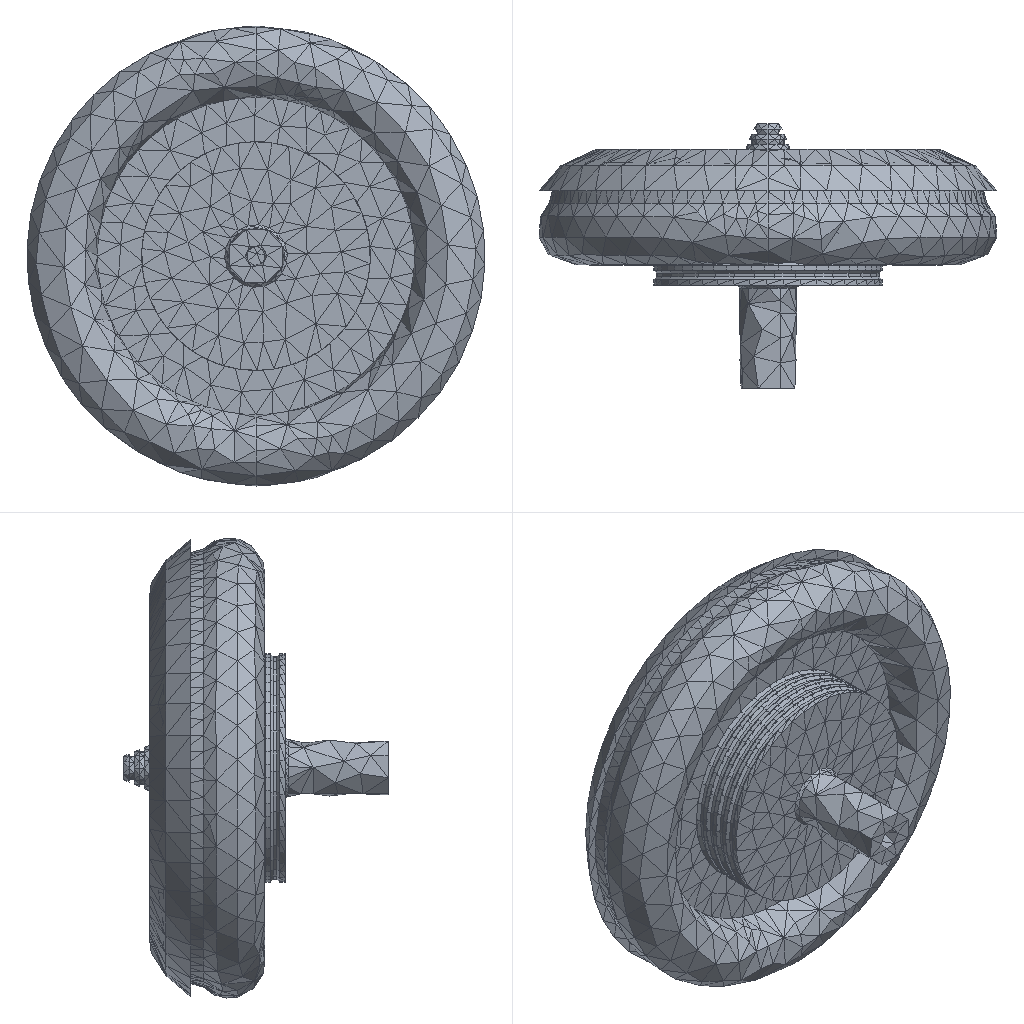Simulation study | ansys workbench
Set-up summary:
category,name,step,type,value,unit,region
solver,ansys_workbench
units,mm-N-s-tonne (MPa),,stated,"/units,MPA"
analysis,LS1,,modal,method=lanb; n_modes=16
load_step,LS1,LS1,modal
mesh,nodes,,,33011
mesh,elements,,,20069
element_type,SOLID187,,,10384
element_type,TARGE170,,,3950
element_type,CONTA174,,,3950
element_type,SOLID186,,,1785
material,Structural Steel,,E,200000,tonne s^-2 mm^-1
material,Structural Steel,,nu,0.3
material,Structural Steel,,density,7.85e-09,tonne mm^-3
material,Structural Steel,,conductivity,60.5,tonne mm s^-3 C^-1
material,Structural Steel,,specific_heat,4.34e+08,mm^2 s^-2 C^-1
material,Structural Steel,,cte,1.2e-05,C^-1
material,Structural Steel,,permeability,10000
material,Structural Steel,,resistivity,0.00017,ohm mm
bc,Fixed Supports,model,fixed,[dofs=ALL],,_FIXEDSU
contact,Contact Region,,bonded (always),element=CONTA174
contact,Contact Region 2,,bonded (always),element=CONTA174
contact,Contact Region 3,,bonded (always),element=CONTA174
contact,Contact Region 4,,bonded (always),element=CONTA174
contact,Contact Region 5,,bonded (always),element=CONTA174
contact,Contact Region 6,,bonded (always),element=CONTA174
contact,Contact Region 7,,bonded (always),element=CONTA174
contact,Contact Region 8,,bonded (always),element=CONTA174
contact,Contact Region 9,,bonded (always),element=CONTA174
contact,Contact Region 10,,bonded (always),element=CONTA174
contact,Contact Region 11,,bonded (always),element=CONTA174
contact,Contact Region 12,,bonded (always),element=CONTA174
contact,Contact Region 13,,bonded (always),element=CONTA174
contact,Contact Region 14,,bonded (always),element=CONTA174
contact,Contact Region 15,,bonded (always),element=CONTA174
contact,Contact Region 16,,bonded (always),element=CONTA174
contact,Contact Region 17,,bonded (always),element=CONTA174
contact,Contact Region 18,,bonded (always),element=CONTA174
contact,Contact Region 19,,bonded (always),element=CONTA174
named_set,_FIXEDSU,,node,71
Ansys APDL input file, long lists of numbers shortened:
/batch
/config,noeldb,1     ! force off writing results to database
*get,_wallstrt,active,,time,wall
! ANSYS input file written by Workbench version 2022 R1
! File used for geometry attach:
/title,wbnew--__ (B5)
! ****** Begin Custom Load Command Snippet ******
/COM, ACT Extensions:
/COM,     LSDYNA, 2021.1
/COM,
! ****** End   Custom Load Command Snippet ******
*DIM,_wb_ProjectScratch_dir,string,248
_wb_ProjectScratch_dir(1) = ''
*DIM,_wb_SolverFiles_dir,string,248
_wb_SolverFiles_dir(1) = ''
*DIM,_wb_userfiles_dir,string,248
_wb_userfiles_dir(1) = ''
/com,--- Data in consistent NMM units. See Solving Units in the help system for more information.
/units,MPA
/nopr
/wb,file,start              !  signify a WB generated input file
/prep7
! Turn off shape checking because checks already performed inside WB mesher.
! See help system for more information.
SHPP,OFF,,NOWARN
/nolist
etcon,set             ! allow ANSYS to choose best KEYOP's for 180x elements, resets any applicable keyopt to MAPDL defaults
/com,*********** Nodes for the whole assembly ***********
nblock,3,,36312
(1i9,3e20.9e3)
        1     2.699417461E+01    -7.691078990E-01    -9.444787595E+01
! (33010 more lines like these left out)
-1
/wb,elem,start            !  set before creation of elements
/com,*********** Elements for Body 1 "___|__2" ***********
et,1,187
eblock,19,solid,,7427
(19i9)
        1        1        1        1        0        0        0        0       10        0     4743    19564    19845    19601    19811    28998    29176    28996    28997
! (14853 more lines like these left out)
-1
/com,*********** Elements for Body 2 "___|__2" ***********
et,2,187
eblock,19,solid,,2220
(19i9)
        2        2        2        2        0        0        0        0       10        0     2523    13536    13544    14294    13986    14611    14693    14618    14615
! (4439 more lines like these left out)
-1
/com,*********** Elements for Body 3 "___|__1" ***********
et,3,186
keyo,3,2,1          ! set full integration on SOLID186
eblock,19,solid,,258
(19i9)
        3        3        3        3        0        0        0        0       20        0     1811     8425     8725     8738     8460     8607     8736     8737     8572
! (515 more lines like these left out)
-1
/com,*********** Elements for Body 4 "___|__1[2]" ***********
et,4,186
keyo,4,2,1          ! set full integration on SOLID186
eblock,19,solid,,258
(19i9)
        4        4        4        4        0        0        0        0       20        0      965     3380     3680     3693     3415     3562     3691     3692     3527
! (515 more lines like these left out)
-1
/com,*********** Elements for Body 5 "___|__1[3]" ***********
et,5,186
keyo,5,2,1          ! set full integration on SOLID186
eblock,19,solid,,258
(19i9)
        5        5        5        5        0        0        0        0       20        0     1553     6904     7204     7217     6939     7086     7215     7216     7051
! (515 more lines like these left out)
-1
/com,*********** Elements for Body 6 "___|__1[4]" ***********
et,6,186
keyo,6,2,1          ! set full integration on SOLID186
eblock,19,solid,,258
(19i9)
        6        6        6        6        0        0        0        0       20        0     1295     5383     5683     5696     5418     5565     5694     5695     5530
! (515 more lines like these left out)
-1
/com,*********** Elements for Body 7 "___|__-__1" ***********
et,7,186
keyo,7,2,1          ! set full integration on SOLID186
eblock,19,solid,,227
(19i9)
        7        7        7        7        0        0        0        0       20        0        1       73      190      181      111      308      191      200      270
! (453 more lines like these left out)
-1
/com,*********** Elements for Body 8 "___|__-__1[2]" ***********
et,8,186
keyo,8,2,1          ! set full integration on SOLID186
eblock,19,solid,,227
(19i9)
        8        8        8        8        0        0        0        0       20        0     2296    11792    11909    11900    11830    12027    11910    11919    11989
! (453 more lines like these left out)
-1
/com,*********** Elements for Body 9 "___|__-__1[3]" ***********
et,9,186
keyo,9,2,1          ! set full integration on SOLID186
eblock,19,solid,,227
(19i9)
        9        9        9        9        0        0        0        0       20        0     2069    10018    10135    10126    10056    10253    10136    10145    10215
! (453 more lines like these left out)
-1
/com,*********** Elements for Body 10 "__|__1" ***********
et,10,187
eblock,19,solid,,737
(19i9)
       10       10       10       10        0        0        0        0       10        0      228     1781     1981     2061     2059     2120     3118     2122     2121
! (1473 more lines like these left out)
-1
/com,*********** Elements for Body 11 "____|__-__1" ***********
et,11,186
keyo,11,2,1          ! set full integration on SOLID186
eblock,19,solid,,72
(19i9)
       11       11       11       11        0        0        0        0       20        0     1223     4971     5035     5034     4972     4980     5038     5039     4981
! (143 more lines like these left out)
-1
/wb,elem,end               !  done creating elements
/com,*********** Send User Defined Coordinate System(s) ***********
csys,0
toffst,273.15,  ! Temperature offset from absolute zero
/com,*********** Set Reference Temperature ***********
tref,22.
/wb,mat,start              !  starting to send materials
/com,*********** Send Materials ***********
Temperature = 'TEMP' ! Temperature
MP,DENS,1,7.85e-09,	! tonne mm^-3
MP,ALPX,1,1.2e-05,	! C^-1
MP,C,1,434000000,	! mm^2 s^-2 C^-1
MP,KXX,1,60.5,	! tonne mm s^-3 C^-1
MP,RSVX,1,0.00017,	! ohm mm
MP,EX,1,200000,	! tonne s^-2 mm^-1
MP,NUXY,1,0.3,
MP,MURX,1,10000,
Temperature = 'TEMP' ! Temperature
MP,DENS,2,7.85e-09,	! tonne mm^-3
MP,ALPX,2,1.2e-05,	! C^-1
MP,C,2,434000000,	! mm^2 s^-2 C^-1
MP,KXX,2,60.5,	! tonne mm s^-3 C^-1
MP,RSVX,2,0.00017,	! ohm mm
MP,EX,2,200000,	! tonne s^-2 mm^-1
MP,NUXY,2,0.3,
MP,MURX,2,10000,
Temperature = 'TEMP' ! Temperature
MP,DENS,3,7.85e-09,	! tonne mm^-3
MP,ALPX,3,1.2e-05,	! C^-1
MP,C,3,434000000,	! mm^2 s^-2 C^-1
MP,KXX,3,60.5,	! tonne mm s^-3 C^-1
MP,RSVX,3,0.00017,	! ohm mm
MP,EX,3,200000,	! tonne s^-2 mm^-1
MP,NUXY,3,0.3,
MP,MURX,3,10000,
Temperature = 'TEMP' ! Temperature
MP,DENS,4,7.85e-09,	! tonne mm^-3
MP,ALPX,4,1.2e-05,	! C^-1
MP,C,4,434000000,	! mm^2 s^-2 C^-1
MP,KXX,4,60.5,	! tonne mm s^-3 C^-1
MP,RSVX,4,0.00017,	! ohm mm
MP,EX,4,200000,	! tonne s^-2 mm^-1
MP,NUXY,4,0.3,
MP,MURX,4,10000,
Temperature = 'TEMP' ! Temperature
MP,DENS,5,7.85e-09,	! tonne mm^-3
MP,ALPX,5,1.2e-05,	! C^-1
MP,C,5,434000000,	! mm^2 s^-2 C^-1
MP,KXX,5,60.5,	! tonne mm s^-3 C^-1
MP,RSVX,5,0.00017,	! ohm mm
MP,EX,5,200000,	! tonne s^-2 mm^-1
MP,NUXY,5,0.3,
MP,MURX,5,10000,
Temperature = 'TEMP' ! Temperature
MP,DENS,6,7.85e-09,	! tonne mm^-3
MP,ALPX,6,1.2e-05,	! C^-1
MP,C,6,434000000,	! mm^2 s^-2 C^-1
MP,KXX,6,60.5,	! tonne mm s^-3 C^-1
MP,RSVX,6,0.00017,	! ohm mm
MP,EX,6,200000,	! tonne s^-2 mm^-1
MP,NUXY,6,0.3,
MP,MURX,6,10000,
Temperature = 'TEMP' ! Temperature
MP,DENS,7,7.85e-09,	! tonne mm^-3
MP,ALPX,7,1.2e-05,	! C^-1
MP,C,7,434000000,	! mm^2 s^-2 C^-1
MP,KXX,7,60.5,	! tonne mm s^-3 C^-1
MP,RSVX,7,0.00017,	! ohm mm
MP,EX,7,200000,	! tonne s^-2 mm^-1
MP,NUXY,7,0.3,
MP,MURX,7,10000,
Temperature = 'TEMP' ! Temperature
MP,DENS,8,7.85e-09,	! tonne mm^-3
MP,ALPX,8,1.2e-05,	! C^-1
MP,C,8,434000000,	! mm^2 s^-2 C^-1
MP,KXX,8,60.5,	! tonne mm s^-3 C^-1
MP,RSVX,8,0.00017,	! ohm mm
MP,EX,8,200000,	! tonne s^-2 mm^-1
MP,NUXY,8,0.3,
MP,MURX,8,10000,
Temperature = 'TEMP' ! Temperature
MP,DENS,9,7.85e-09,	! tonne mm^-3
MP,ALPX,9,1.2e-05,	! C^-1
MP,C,9,434000000,	! mm^2 s^-2 C^-1
MP,KXX,9,60.5,	! tonne mm s^-3 C^-1
MP,RSVX,9,0.00017,	! ohm mm
MP,EX,9,200000,	! tonne s^-2 mm^-1
MP,NUXY,9,0.3,
MP,MURX,9,10000,
Temperature = 'TEMP' ! Temperature
MP,DENS,10,7.85e-09,	! tonne mm^-3
MP,ALPX,10,1.2e-05,	! C^-1
MP,C,10,434000000,	! mm^2 s^-2 C^-1
MP,KXX,10,60.5,	! tonne mm s^-3 C^-1
MP,RSVX,10,0.00017,	! ohm mm
MP,EX,10,200000,	! tonne s^-2 mm^-1
MP,NUXY,10,0.3,
MP,MURX,10,10000,
Temperature = 'TEMP' ! Temperature
MP,DENS,11,7.85e-09,	! tonne mm^-3
MP,ALPX,11,1.2e-05,	! C^-1
MP,C,11,434000000,	! mm^2 s^-2 C^-1
MP,KXX,11,60.5,	! tonne mm s^-3 C^-1
MP,RSVX,11,0.00017,	! ohm mm
MP,EX,11,200000,	! tonne s^-2 mm^-1
MP,NUXY,11,0.3,
MP,MURX,11,10000,
/wb,mat,end                !  done sending materials
!************************* Model Summary ********************
!___|__2,	结构钢,	matid,	1
!___|__2,	结构钢,	matid,	2
!___|__1,	结构钢,	matid,	3
!___|__1[2],	结构钢,	matid,	4
!___|__1[3],	结构钢,	matid,	5
!___|__1[4],	结构钢,	matid,	6
!___|__-__1,	结构钢,	matid,	7
!___|__-__1[2],	结构钢,	matid,	8
!___|__-__1[3],	结构钢,	matid,	9
!__|__1,	结构钢,	matid,	10
!____|__-__1,	结构钢,	matid,	11
!************************* End Model Summary ********************
! get the diagonal of the bounding box. Needed later for other things
*get,_xmin,node,,mnloc,x
*get,_ymin,node,,mnloc,y
*get,_zmin,node,,mnloc,z
*get,_xmax,node,,mxloc,x
*get,_ymax,node,,mxloc,y
*get,_zmax,node,,mxloc,z
_ASMDIAG=(_xmax-_xmin)*(_xmax-_xmin)+(_ymax-_ymin)*(_ymax-_ymin)+(_zmax-_zmin)*(_zmax-_zmin)
_ASMDIAG=SQRT(_ASMDIAG)
/wb,contact,start          !  starting to send contact
/com,*********** Create Contact "接触区域" ***********
/com,            Real Constant Set For Above Contact Is 13 & 12
*set,tid,13
*set,cid,12
r,tid
r,cid
et,tid,170
et,cid,174
eblock,10,,,481
(15i9)
    22252       13       13       13        0    18309    18380    18379    18379    22461    23015    18379    22460
! (480 more lines like these left out)
-1
eblock,10,,,481
(15i9)
    22733       12       12       12        0    18309    18380    18379    18379    22461    23015    18379    22460
! (480 more lines like these left out)
-1
eblock,10,,,416
(15i9)
    23214       12       13       12        0    13892    14063    13906    13906    16688    16776    13906    16685
! (415 more lines like these left out)
-1
eblock,10,,,416
(15i9)
    23630       13       12       13        0    13892    14063    13906    13906    16688    16776    13906    16685
! (415 more lines like these left out)
-1
keyo,cid,8,2               ! auto create asymmetric contact (from Program Controlled setting)
keyo,cid,10,0              ! adjust contact stiffness each NR iteration (from Program Controlled setting)
keyo,cid,12,5              ! bonded always
keyo,cid,18,1              ! small sliding turned on by application
keyo,cid,2,0               ! augmented Lagrange (from Program Controlled setting)
keyo,cid,4,0               ! on Gauss point (from Program Controlled setting)
keyo,cid,9,1               ! ignore initial gaps/penetration
keyo,cid,7,0               ! No Prediction
rmod,tid,3,10.      ! FKN
rmod,tid,5,0.       ! ICONT
rmod,tid,6,0.       ! PINB
rmod,tid,10,0.      ! CNOF
rmod,tid,12,0.      ! FKT
rmod,tid,36,56      ! WB DSID
rmod,cid,3,10.      ! FKN
rmod,cid,5,0.       ! ICONT
rmod,cid,6,0.       ! PINB
rmod,cid,10,0.      ! CNOF
rmod,cid,12,0.      ! FKT
rmod,cid,36,56      ! WB DSID
/com,*********** Create Contact "接触区域 2" ***********
/com,            Real Constant Set For Above Contact Is 15 & 14
*set,tid,15
*set,cid,14
r,tid
r,cid
et,tid,170
et,cid,174
eblock,10,,,185
(15i9)
    24046       15       15       15        0    19951    20008    19985    19985    30704    30941    19985    30701
! (184 more lines like these left out)
-1
eblock,10,,,185
(15i9)
    24231       14       14       14        0    19951    20008    19985    19985    30704    30941    19985    30701
! (184 more lines like these left out)
-1
eblock,10,,,86
(15i9)
    24416       14       15       14        0     5529     5558     5557     5557     6360     6427     5557     6359
! (85 more lines like these left out)
-1
eblock,10,,,86
(15i9)
    24502       15       14       15        0     5529     5558     5557     5557     6360     6427     5557     6359
! (85 more lines like these left out)
-1
keyo,cid,8,2               ! auto create asymmetric contact (from Program Controlled setting)
keyo,cid,10,0              ! adjust contact stiffness each NR iteration (from Program Controlled setting)
keyo,cid,12,5              ! bonded always
keyo,cid,18,1              ! small sliding turned on by application
keyo,cid,2,0               ! augmented Lagrange (from Program Controlled setting)
keyo,cid,4,0               ! on Gauss point (from Program Controlled setting)
keyo,cid,9,1               ! ignore initial gaps/penetration
keyo,cid,7,0               ! No Prediction
rmod,tid,3,10.      ! FKN
rmod,tid,5,0.       ! ICONT
rmod,tid,6,0.       ! PINB
rmod,tid,10,0.      ! CNOF
rmod,tid,12,0.      ! FKT
rmod,tid,36,59      ! WB DSID
rmod,cid,3,10.      ! FKN
rmod,cid,5,0.       ! ICONT
rmod,cid,6,0.       ! PINB
rmod,cid,10,0.      ! CNOF
rmod,cid,12,0.      ! FKT
rmod,cid,36,59      ! WB DSID
/com,*********** Create Contact "接触区域 3" ***********
/com,            Real Constant Set For Above Contact Is 17 & 16
*set,tid,17
*set,cid,16
r,tid
r,cid
et,tid,170
et,cid,174
eblock,10,,,34
(15i9)
    24588       17       17       17        0    19964    20040    20025    20025    30799    31096    20025    30797
! (33 more lines like these left out)
-1
eblock,10,,,34
(15i9)
    24622       16       16       16        0    19964    20040    20025    20025    30799    31096    20025    30797
! (33 more lines like these left out)
-1
eblock,10,,,12
(15i9)
    24656       16       17       16        0     1941     1797     1796     1796     2209     2201     1796     2205
! (11 more lines like these left out)
-1
eblock,10,,,12
(15i9)
    24668       17       16       17        0     1941     1797     1796     1796     2209     2201     1796     2205
! (11 more lines like these left out)
-1
keyo,cid,8,2               ! auto create asymmetric contact (from Program Controlled setting)
keyo,cid,10,0              ! adjust contact stiffness each NR iteration (from Program Controlled setting)
keyo,cid,12,5              ! bonded always
keyo,cid,18,1              ! small sliding turned on by application
keyo,cid,2,0               ! augmented Lagrange (from Program Controlled setting)
keyo,cid,4,0               ! on Gauss point (from Program Controlled setting)
keyo,cid,9,1               ! ignore initial gaps/penetration
keyo,cid,7,0               ! No Prediction
rmod,tid,3,10.      ! FKN
rmod,tid,5,0.       ! ICONT
rmod,tid,6,0.       ! PINB
rmod,tid,10,0.      ! CNOF
rmod,tid,12,0.      ! FKT
rmod,tid,36,62      ! WB DSID
rmod,cid,3,10.      ! FKN
rmod,cid,5,0.       ! ICONT
rmod,cid,6,0.       ! PINB
rmod,cid,10,0.      ! CNOF
rmod,cid,12,0.      ! FKT
rmod,cid,36,62      ! WB DSID
/com,*********** Create Contact "接触区域 4" ***********
/com,            Real Constant Set For Above Contact Is 19 & 18
*set,tid,19
*set,cid,18
r,tid
r,cid
et,tid,170
et,cid,174
eblock,10,,,61
(15i9)
    24680       19       19       19        0    19957    20025    20027    20027    30748    31095    20027    30749
! (60 more lines like these left out)
-1
eblock,10,,,61
(15i9)
    24741       18       18       18        0    19957    20025    20027    20027    30748    31095    20027    30749
! (60 more lines like these left out)
-1
eblock,10,,,18
(15i9)
    24802       18       19       18        0     4982     4981     5039     5039     5285     5286     5039     5288
! (17 more lines like these left out)
-1
eblock,10,,,18
(15i9)
    24820       19       18       19        0     4982     4981     5039     5039     5285     5286     5039     5288
! (17 more lines like these left out)
-1
keyo,cid,8,2               ! auto create asymmetric contact (from Program Controlled setting)
keyo,cid,10,0              ! adjust contact stiffness each NR iteration (from Program Controlled setting)
keyo,cid,12,5              ! bonded always
keyo,cid,18,1              ! small sliding turned on by application
keyo,cid,2,0               ! augmented Lagrange (from Program Controlled setting)
keyo,cid,4,0               ! on Gauss point (from Program Controlled setting)
keyo,cid,9,1               ! ignore initial gaps/penetration
keyo,cid,7,0               ! No Prediction
rmod,tid,3,10.      ! FKN
rmod,tid,5,0.       ! ICONT
rmod,tid,6,0.       ! PINB
rmod,tid,10,0.      ! CNOF
rmod,tid,12,0.      ! FKT
rmod,tid,36,65      ! WB DSID
rmod,cid,3,10.      ! FKN
rmod,cid,5,0.       ! ICONT
rmod,cid,6,0.       ! PINB
rmod,cid,10,0.      ! CNOF
rmod,cid,12,0.      ! FKT
rmod,cid,36,65      ! WB DSID
/com,*********** Create Contact "接触区域 5" ***********
/com,            Real Constant Set For Above Contact Is 21 & 20
*set,tid,21
*set,cid,20
r,tid
r,cid
et,tid,170
et,cid,174
eblock,10,,,86
(15i9)
    24838       21       21       21        0     8571     8600     8599     8599     9402     9469     8599     9401
! (85 more lines like these left out)
-1
eblock,10,,,86
(15i9)
    24924       20       20       20        0     8571     8600     8599     8599     9402     9469     8599     9401
! (85 more lines like these left out)
-1
eblock,10,,,227
(15i9)
    25010       20       21       20        0       73      111      181      190      827      981     1121      830
! (226 more lines like these left out)
-1
eblock,10,,,227
(15i9)
    25237       21       20       21        0       73      111      181      190      827      981     1121      830
! (226 more lines like these left out)
-1
keyo,cid,8,2               ! auto create asymmetric contact (from Program Controlled setting)
keyo,cid,10,0              ! adjust contact stiffness each NR iteration (from Program Controlled setting)
keyo,cid,12,5              ! bonded always
keyo,cid,18,1              ! small sliding turned on by application
keyo,cid,2,0               ! augmented Lagrange (from Program Controlled setting)
keyo,cid,4,0               ! on Gauss point (from Program Controlled setting)
keyo,cid,9,1               ! ignore initial gaps/penetration
keyo,cid,7,0               ! No Prediction
rmod,tid,3,10.      ! FKN
rmod,tid,5,0.       ! ICONT
rmod,tid,6,0.       ! PINB
rmod,tid,10,0.      ! CNOF
rmod,tid,12,0.      ! FKT
rmod,tid,36,68      ! WB DSID
rmod,cid,3,10.      ! FKN
rmod,cid,5,0.       ! ICONT
rmod,cid,6,0.       ! PINB
rmod,cid,10,0.      ! CNOF
rmod,cid,12,0.      ! FKT
rmod,cid,36,68      ! WB DSID
/com,*********** Create Contact "接触区域 6" ***********
/com,            Real Constant Set For Above Contact Is 23 & 22
*set,tid,23
*set,cid,22
r,tid
r,cid
et,tid,170
et,cid,174
eblock,10,,,86
(15i9)
    25464       23       23       23        0     8644     8616     8615     8615     9503     9498     8615     9500
! (85 more lines like these left out)
-1
eblock,10,,,86
(15i9)
    25550       22       22       22        0     8644     8616     8615     8615     9503     9498     8615     9500
! (85 more lines like these left out)
-1
eblock,10,,,227
(15i9)
    25636       22       23       22        0    11919    11989    12027    11910    12886    13094    12858    12856
! (226 more lines like these left out)
-1
eblock,10,,,227
(15i9)
    25863       23       22       23        0    11919    11989    12027    11910    12886    13094    12858    12856
! (226 more lines like these left out)
-1
keyo,cid,8,2               ! auto create asymmetric contact (from Program Controlled setting)
keyo,cid,10,0              ! adjust contact stiffness each NR iteration (from Program Controlled setting)
keyo,cid,12,5              ! bonded always
keyo,cid,18,1              ! small sliding turned on by application
keyo,cid,2,0               ! augmented Lagrange (from Program Controlled setting)
keyo,cid,4,0               ! on Gauss point (from Program Controlled setting)
keyo,cid,9,1               ! ignore initial gaps/penetration
keyo,cid,7,0               ! No Prediction
rmod,tid,3,10.      ! FKN
rmod,tid,5,0.       ! ICONT
rmod,tid,6,0.       ! PINB
rmod,tid,10,0.      ! CNOF
rmod,tid,12,0.      ! FKT
rmod,tid,36,71      ! WB DSID
rmod,cid,3,10.      ! FKN
rmod,cid,5,0.       ! ICONT
rmod,cid,6,0.       ! PINB
rmod,cid,10,0.      ! CNOF
rmod,cid,12,0.      ! FKT
rmod,cid,36,71      ! WB DSID
/com,*********** Create Contact "接触区域 7" ***********
/com,            Real Constant Set For Above Contact Is 25 & 24
*set,tid,25
*set,cid,24
r,tid
r,cid
et,tid,170
et,cid,174
eblock,10,,,36
(15i9)
    26090       25       25       25        0     8740     8721     8731     8732     9766     9765     9790     9792
! (35 more lines like these left out)
-1
eblock,10,,,36
(15i9)
    26126       24       24       24        0     8740     8721     8731     8732     9766     9765     9790     9792
! (35 more lines like these left out)
-1
eblock,10,,,54
(15i9)
    26162       24       25       24        0     4990     4953     4914     4913     5203     5087     5083     5085
! (53 more lines like these left out)
-1
eblock,10,,,54
(15i9)
    26216       25       24       25        0     4990     4953     4914     4913     5203     5087     5083     5085
! (53 more lines like these left out)
-1
keyo,cid,8,2               ! auto create asymmetric contact (from Program Controlled setting)
keyo,cid,10,0              ! adjust contact stiffness each NR iteration (from Program Controlled setting)
keyo,cid,12,5              ! bonded always
keyo,cid,18,1              ! small sliding turned on by application
keyo,cid,2,0               ! augmented Lagrange (from Program Controlled setting)
keyo,cid,4,0               ! on Gauss point (from Program Controlled setting)
keyo,cid,9,1               ! ignore initial gaps/penetration
keyo,cid,7,0               ! No Prediction
rmod,tid,3,10.      ! FKN
rmod,tid,5,0.       ! ICONT
rmod,tid,6,0.       ! PINB
rmod,tid,10,0.      ! CNOF
rmod,tid,12,0.      ! FKT
rmod,tid,36,74      ! WB DSID
rmod,cid,3,10.      ! FKN
rmod,cid,5,0.       ! ICONT
rmod,cid,6,0.       ! PINB
rmod,cid,10,0.      ! CNOF
rmod,cid,12,0.      ! FKT
rmod,cid,36,74      ! WB DSID
/com,*********** Create Contact "接触区域 8" ***********
/com,            Real Constant Set For Above Contact Is 27 & 26
*set,tid,27
*set,cid,26
r,tid
r,cid
et,tid,170
et,cid,174
eblock,10,,,86
(15i9)
    26270       27       27       27        0     3526     3555     3554     3554     4357     4424     3554     4356
! (85 more lines like these left out)
-1
eblock,10,,,86
(15i9)
    26356       26       26       26        0     3526     3555     3554     3554     4357     4424     3554     4356
! (85 more lines like these left out)
-1
eblock,10,,,227
(15i9)
    26442       26       27       26        0    11792    11830    11900    11909    12546    12700    12840    12549
! (226 more lines like these left out)
-1
eblock,10,,,227
(15i9)
    26669       27       26       27        0    11792    11830    11900    11909    12546    12700    12840    12549
! (226 more lines like these left out)
-1
keyo,cid,8,2               ! auto create asymmetric contact (from Program Controlled setting)
keyo,cid,10,0              ! adjust contact stiffness each NR iteration (from Program Controlled setting)
keyo,cid,12,5              ! bonded always
keyo,cid,18,1              ! small sliding turned on by application
keyo,cid,2,0               ! augmented Lagrange (from Program Controlled setting)
keyo,cid,4,0               ! on Gauss point (from Program Controlled setting)
keyo,cid,9,1               ! ignore initial gaps/penetration
keyo,cid,7,0               ! No Prediction
rmod,tid,3,10.      ! FKN
rmod,tid,5,0.       ! ICONT
rmod,tid,6,0.       ! PINB
rmod,tid,10,0.      ! CNOF
rmod,tid,12,0.      ! FKT
rmod,tid,36,77      ! WB DSID
rmod,cid,3,10.      ! FKN
rmod,cid,5,0.       ! ICONT
rmod,cid,6,0.       ! PINB
rmod,cid,10,0.      ! CNOF
rmod,cid,12,0.      ! FKT
rmod,cid,36,77      ! WB DSID
/com,*********** Create Contact "接触区域 9" ***********
/com,            Real Constant Set For Above Contact Is 29 & 28
*set,tid,29
*set,cid,28
r,tid
r,cid
et,tid,170
et,cid,174
eblock,10,,,86
(15i9)
    26896       29       29       29        0     3599     3571     3570     3570     4458     4453     3570     4455
! (85 more lines like these left out)
-1
eblock,10,,,86
(15i9)
    26982       28       28       28        0     3599     3571     3570     3570     4458     4453     3570     4455
! (85 more lines like these left out)
-1
eblock,10,,,96
(15i9)
    27068       28       29       28        0     1798     1990     1803     1803     2222     2275     1803     2214
! (95 more lines like these left out)
-1
eblock,10,,,96
(15i9)
    27164       29       28       29        0     1798     1990     1803     1803     2222     2275     1803     2214
! (95 more lines like these left out)
-1
keyo,cid,8,2               ! auto create asymmetric contact (from Program Controlled setting)
keyo,cid,10,0              ! adjust contact stiffness each NR iteration (from Program Controlled setting)
keyo,cid,12,5              ! bonded always
keyo,cid,18,1              ! small sliding turned on by application
keyo,cid,2,0               ! augmented Lagrange (from Program Controlled setting)
keyo,cid,4,0               ! on Gauss point (from Program Controlled setting)
keyo,cid,9,1               ! ignore initial gaps/penetration
keyo,cid,7,0               ! No Prediction
rmod,tid,3,10.      ! FKN
rmod,tid,5,0.       ! ICONT
rmod,tid,6,0.       ! PINB
rmod,tid,10,0.      ! CNOF
rmod,tid,12,0.      ! FKT
rmod,tid,36,80      ! WB DSID
rmod,cid,3,10.      ! FKN
rmod,cid,5,0.       ! ICONT
rmod,cid,6,0.       ! PINB
rmod,cid,10,0.      ! CNOF
rmod,cid,12,0.      ! FKT
rmod,cid,36,80      ! WB DSID
/com,*********** Create Contact "接触区域 10" ***********
/com,            Real Constant Set For Above Contact Is 31 & 30
*set,tid,31
*set,cid,30
r,tid
r,cid
et,tid,170
et,cid,174
eblock,10,,,36
(15i9)
    27260       31       31       31        0     3695     3676     3686     3687     4721     4720     4745     4747
! (35 more lines like these left out)
-1
eblock,10,,,36
(15i9)
    27296       30       30       30        0     3695     3676     3686     3687     4721     4720     4745     4747
! (35 more lines like these left out)
-1
eblock,10,,,36
(15i9)
    27332       30       31       30        0     4990     4953     4914     4913     5203     5087     5083     5085
! (35 more lines like these left out)
-1
eblock,10,,,36
(15i9)
    27368       31       30       31        0     4990     4953     4914     4913     5203     5087     5083     5085
! (35 more lines like these left out)
-1
keyo,cid,8,2               ! auto create asymmetric contact (from Program Controlled setting)
keyo,cid,10,0              ! adjust contact stiffness each NR iteration (from Program Controlled setting)
keyo,cid,12,5              ! bonded always
keyo,cid,18,1              ! small sliding turned on by application
keyo,cid,2,0               ! augmented Lagrange (from Program Controlled setting)
keyo,cid,4,0               ! on Gauss point (from Program Controlled setting)
keyo,cid,9,1               ! ignore initial gaps/penetration
keyo,cid,7,0               ! No Prediction
rmod,tid,3,10.      ! FKN
rmod,tid,5,0.       ! ICONT
rmod,tid,6,0.       ! PINB
rmod,tid,10,0.      ! CNOF
rmod,tid,12,0.      ! FKT
rmod,tid,36,83      ! WB DSID
rmod,cid,3,10.      ! FKN
rmod,cid,5,0.       ! ICONT
rmod,cid,6,0.       ! PINB
rmod,cid,10,0.      ! CNOF
rmod,cid,12,0.      ! FKT
rmod,cid,36,83      ! WB DSID
/com,*********** Create Contact "接触区域 11" ***********
/com,            Real Constant Set For Above Contact Is 33 & 32
*set,tid,33
*set,cid,32
r,tid
r,cid
et,tid,170
et,cid,174
eblock,10,,,86
(15i9)
    27404       33       33       33        0     7123     7095     7094     7094     7982     7977     7094     7979
! (85 more lines like these left out)
-1
eblock,10,,,86
(15i9)
    27490       32       32       32        0     7123     7095     7094     7094     7982     7977     7094     7979
! (85 more lines like these left out)
-1
eblock,10,,,227
(15i9)
    27576       32       33       32        0      200      270      308      191     1167     1375     1139     1137
! (226 more lines like these left out)
-1
eblock,10,,,227
(15i9)
    27803       33       32       33        0      200      270      308      191     1167     1375     1139     1137
! (226 more lines like these left out)
-1
keyo,cid,8,2               ! auto create asymmetric contact (from Program Controlled setting)
keyo,cid,10,0              ! adjust contact stiffness each NR iteration (from Program Controlled setting)
keyo,cid,12,5              ! bonded always
keyo,cid,18,1              ! small sliding turned on by application
keyo,cid,2,0               ! augmented Lagrange (from Program Controlled setting)
keyo,cid,4,0               ! on Gauss point (from Program Controlled setting)
keyo,cid,9,1               ! ignore initial gaps/penetration
keyo,cid,7,0               ! No Prediction
rmod,tid,3,10.      ! FKN
rmod,tid,5,0.       ! ICONT
rmod,tid,6,0.       ! PINB
rmod,tid,10,0.      ! CNOF
rmod,tid,12,0.      ! FKT
rmod,tid,36,86      ! WB DSID
rmod,cid,3,10.      ! FKN
rmod,cid,5,0.       ! ICONT
rmod,cid,6,0.       ! PINB
rmod,cid,10,0.      ! CNOF
rmod,cid,12,0.      ! FKT
rmod,cid,36,86      ! WB DSID
/com,*********** Create Contact "接触区域 12" ***********
/com,            Real Constant Set For Above Contact Is 35 & 34
*set,tid,35
*set,cid,34
r,tid
r,cid
et,tid,170
et,cid,174
eblock,10,,,86
(15i9)
    28030       35       35       35        0     7050     7079     7078     7078     7881     7948     7078     7880
! (85 more lines like these left out)
-1
eblock,10,,,86
(15i9)
    28116       34       34       34        0     7050     7079     7078     7078     7881     7948     7078     7880
! (85 more lines like these left out)
-1
eblock,10,,,227
(15i9)
    28202       34       35       34        0    10018    10056    10126    10135    10772    10926    11066    10775
! (226 more lines like these left out)
-1
eblock,10,,,227
(15i9)
    28429       35       34       35        0    10018    10056    10126    10135    10772    10926    11066    10775
! (226 more lines like these left out)
-1
keyo,cid,8,2               ! auto create asymmetric contact (from Program Controlled setting)
keyo,cid,10,0              ! adjust contact stiffness each NR iteration (from Program Controlled setting)
keyo,cid,12,5              ! bonded always
keyo,cid,18,1              ! small sliding turned on by application
keyo,cid,2,0               ! augmented Lagrange (from Program Controlled setting)
keyo,cid,4,0               ! on Gauss point (from Program Controlled setting)
keyo,cid,9,1               ! ignore initial gaps/penetration
keyo,cid,7,0               ! No Prediction
rmod,tid,3,10.      ! FKN
rmod,tid,5,0.       ! ICONT
rmod,tid,6,0.       ! PINB
rmod,tid,10,0.      ! CNOF
rmod,tid,12,0.      ! FKT
rmod,tid,36,89      ! WB DSID
rmod,cid,3,10.      ! FKN
rmod,cid,5,0.       ! ICONT
rmod,cid,6,0.       ! PINB
rmod,cid,10,0.      ! CNOF
rmod,cid,12,0.      ! FKT
rmod,cid,36,89      ! WB DSID
/com,*********** Create Contact "接触区域 13" ***********
/com,            Real Constant Set For Above Contact Is 37 & 36
*set,tid,37
*set,cid,36
r,tid
r,cid
et,tid,170
et,cid,174
eblock,10,,,36
(15i9)
    28656       37       37       37        0     7219     7200     7210     7211     8245     8244     8269     8271
! (35 more lines like these left out)
-1
eblock,10,,,36
(15i9)
    28692       36       36       36        0     7219     7200     7210     7211     8245     8244     8269     8271
! (35 more lines like these left out)
-1
eblock,10,,,54
(15i9)
    28728       36       37       36        0     4991     4961     4953     4990     5228     5202     5203     5302
! (53 more lines like these left out)
-1
eblock,10,,,54
(15i9)
    28782       37       36       37        0     4991     4961     4953     4990     5228     5202     5203     5302
! (53 more lines like these left out)
-1
keyo,cid,8,2               ! auto create asymmetric contact (from Program Controlled setting)
keyo,cid,10,0              ! adjust contact stiffness each NR iteration (from Program Controlled setting)
keyo,cid,12,5              ! bonded always
keyo,cid,18,1              ! small sliding turned on by application
keyo,cid,2,0               ! augmented Lagrange (from Program Controlled setting)
keyo,cid,4,0               ! on Gauss point (from Program Controlled setting)
keyo,cid,9,1               ! ignore initial gaps/penetration
keyo,cid,7,0               ! No Prediction
rmod,tid,3,10.      ! FKN
rmod,tid,5,0.       ! ICONT
rmod,tid,6,0.       ! PINB
rmod,tid,10,0.      ! CNOF
rmod,tid,12,0.      ! FKT
rmod,tid,36,92      ! WB DSID
rmod,cid,3,10.      ! FKN
rmod,cid,5,0.       ! ICONT
rmod,cid,6,0.       ! PINB
rmod,cid,10,0.      ! CNOF
rmod,cid,12,0.      ! FKT
rmod,cid,36,92      ! WB DSID
/com,*********** Create Contact "接触区域 14" ***********
/com,            Real Constant Set For Above Contact Is 39 & 38
*set,tid,39
*set,cid,38
r,tid
r,cid
et,tid,170
et,cid,174
eblock,10,,,86
(15i9)
    28836       39       39       39        0     5602     5574     5573     5573     6461     6456     5573     6458
! (85 more lines like these left out)
-1
eblock,10,,,86
(15i9)
    28922       38       38       38        0     5602     5574     5573     5573     6461     6456     5573     6458
! (85 more lines like these left out)
-1
eblock,10,,,227
(15i9)
    29008       38       39       38        0    10145    10215    10253    10136    11112    11320    11084    11082
! (226 more lines like these left out)
-1
eblock,10,,,227
(15i9)
    29235       39       38       39        0    10145    10215    10253    10136    11112    11320    11084    11082
! (226 more lines like these left out)
-1
keyo,cid,8,2               ! auto create asymmetric contact (from Program Controlled setting)
keyo,cid,10,0              ! adjust contact stiffness each NR iteration (from Program Controlled setting)
keyo,cid,12,5              ! bonded always
keyo,cid,18,1              ! small sliding turned on by application
keyo,cid,2,0               ! augmented Lagrange (from Program Controlled setting)
keyo,cid,4,0               ! on Gauss point (from Program Controlled setting)
keyo,cid,9,1               ! ignore initial gaps/penetration
keyo,cid,7,0               ! No Prediction
rmod,tid,3,10.      ! FKN
rmod,tid,5,0.       ! ICONT
rmod,tid,6,0.       ! PINB
rmod,tid,10,0.      ! CNOF
rmod,tid,12,0.      ! FKT
rmod,tid,36,95      ! WB DSID
rmod,cid,3,10.      ! FKN
rmod,cid,5,0.       ! ICONT
rmod,cid,6,0.       ! PINB
rmod,cid,10,0.      ! CNOF
rmod,cid,12,0.      ! FKT
rmod,cid,36,95      ! WB DSID
/com,*********** Create Contact "接触区域 15" ***********
/com,            Real Constant Set For Above Contact Is 41 & 40
*set,tid,41
*set,cid,40
r,tid
r,cid
et,tid,170
et,cid,174
eblock,10,,,36
(15i9)
    29462       41       41       41        0     5698     5679     5689     5690     6724     6723     6748     6750
! (35 more lines like these left out)
-1
eblock,10,,,36
(15i9)
    29498       40       40       40        0     5698     5679     5689     5690     6724     6723     6748     6750
! (35 more lines like these left out)
-1
eblock,10,,,36
(15i9)
    29534       40       41       40        0     4992     4969     4961     4991     5253     5227     5228     5304
! (35 more lines like these left out)
-1
eblock,10,,,36
(15i9)
    29570       41       40       41        0     4992     4969     4961     4991     5253     5227     5228     5304
! (35 more lines like these left out)
-1
keyo,cid,8,2               ! auto create asymmetric contact (from Program Controlled setting)
keyo,cid,10,0              ! adjust contact stiffness each NR iteration (from Program Controlled setting)
keyo,cid,12,5              ! bonded always
keyo,cid,18,1              ! small sliding turned on by application
keyo,cid,2,0               ! augmented Lagrange (from Program Controlled setting)
keyo,cid,4,0               ! on Gauss point (from Program Controlled setting)
keyo,cid,9,1               ! ignore initial gaps/penetration
keyo,cid,7,0               ! No Prediction
rmod,tid,3,10.      ! FKN
rmod,tid,5,0.       ! ICONT
rmod,tid,6,0.       ! PINB
rmod,tid,10,0.      ! CNOF
rmod,tid,12,0.      ! FKT
rmod,tid,36,98      ! WB DSID
rmod,cid,3,10.      ! FKN
rmod,cid,5,0.       ! ICONT
rmod,cid,6,0.       ! PINB
rmod,cid,10,0.      ! CNOF
rmod,cid,12,0.      ! FKT
rmod,cid,36,98      ! WB DSID
/com,*********** Create Contact "接触区域 16" ***********
/com,            Real Constant Set For Above Contact Is 43 & 42
*set,tid,43
*set,cid,42
r,tid
r,cid
et,tid,170
et,cid,174
eblock,10,,,20
(15i9)
    29606       43       43       43        0      444      445      528      527     1680     1683     1774     1681
! (19 more lines like these left out)
-1
eblock,10,,,20
(15i9)
    29626       42       42       42        0      444      445      528      527     1680     1683     1774     1681
! (19 more lines like these left out)
-1
eblock,10,,,36
(15i9)
    29646       42       43       42        0     4991     4961     4953     4990     5228     5202     5203     5302
! (35 more lines like these left out)
-1
eblock,10,,,36
(15i9)
    29682       43       42       43        0     4991     4961     4953     4990     5228     5202     5203     5302
! (35 more lines like these left out)
-1
keyo,cid,8,2               ! auto create asymmetric contact (from Program Controlled setting)
keyo,cid,10,0              ! adjust contact stiffness each NR iteration (from Program Controlled setting)
keyo,cid,12,5              ! bonded always
keyo,cid,18,1              ! small sliding turned on by application
keyo,cid,2,0               ! augmented Lagrange (from Program Controlled setting)
keyo,cid,4,0               ! on Gauss point (from Program Controlled setting)
keyo,cid,9,1               ! ignore initial gaps/penetration
keyo,cid,7,0               ! No Prediction
rmod,tid,3,10.      ! FKN
rmod,tid,5,0.       ! ICONT
rmod,tid,6,0.       ! PINB
rmod,tid,10,0.      ! CNOF
rmod,tid,12,0.      ! FKT
rmod,tid,36,101     ! WB DSID
rmod,cid,3,10.      ! FKN
rmod,cid,5,0.       ! ICONT
rmod,cid,6,0.       ! PINB
rmod,cid,10,0.      ! CNOF
rmod,cid,12,0.      ! FKT
rmod,cid,36,101     ! WB DSID
/com,*********** Create Contact "接触区域 17" ***********
/com,            Real Constant Set For Above Contact Is 45 & 44
*set,tid,45
*set,cid,44
r,tid
r,cid
et,tid,170
et,cid,174
eblock,10,,,20
(15i9)
    29718       45       45       45        0    12163    12164    12247    12246    13399    13402    13493    13400
! (19 more lines like these left out)
-1
eblock,10,,,20
(15i9)
    29738       44       44       44        0    12163    12164    12247    12246    13399    13402    13493    13400
! (19 more lines like these left out)
-1
eblock,10,,,36
(15i9)
    29758       44       45       44        0     4990     4953     4914     4913     5203     5087     5083     5085
! (35 more lines like these left out)
-1
eblock,10,,,36
(15i9)
    29794       45       44       45        0     4990     4953     4914     4913     5203     5087     5083     5085
! (35 more lines like these left out)
-1
keyo,cid,8,2               ! auto create asymmetric contact (from Program Controlled setting)
keyo,cid,10,0              ! adjust contact stiffness each NR iteration (from Program Controlled setting)
keyo,cid,12,5              ! bonded always
keyo,cid,18,1              ! small sliding turned on by application
keyo,cid,2,0               ! augmented Lagrange (from Program Controlled setting)
keyo,cid,4,0               ! on Gauss point (from Program Controlled setting)
keyo,cid,9,1               ! ignore initial gaps/penetration
keyo,cid,7,0               ! No Prediction
rmod,tid,3,10.      ! FKN
rmod,tid,5,0.       ! ICONT
rmod,tid,6,0.       ! PINB
rmod,tid,10,0.      ! CNOF
rmod,tid,12,0.      ! FKT
rmod,tid,36,104     ! WB DSID
rmod,cid,3,10.      ! FKN
rmod,cid,5,0.       ! ICONT
rmod,cid,6,0.       ! PINB
rmod,cid,10,0.      ! CNOF
rmod,cid,12,0.      ! FKT
rmod,cid,36,104     ! WB DSID
/com,*********** Create Contact "接触区域 18" ***********
/com,            Real Constant Set For Above Contact Is 47 & 46
*set,tid,47
*set,cid,46
r,tid
r,cid
et,tid,170
et,cid,174
eblock,10,,,20
(15i9)
    29830       47       47       47        0    10389    10390    10473    10472    11625    11628    11719    11626
! (19 more lines like these left out)
-1
eblock,10,,,20
(15i9)
    29850       46       46       46        0    10389    10390    10473    10472    11625    11628    11719    11626
! (19 more lines like these left out)
-1
eblock,10,,,36
(15i9)
    29870       46       47       46        0     4992     4969     4961     4991     5253     5227     5228     5304
! (35 more lines like these left out)
-1
eblock,10,,,36
(15i9)
    29906       47       46       47        0     4992     4969     4961     4991     5253     5227     5228     5304
! (35 more lines like these left out)
-1
keyo,cid,8,2               ! auto create asymmetric contact (from Program Controlled setting)
keyo,cid,10,0              ! adjust contact stiffness each NR iteration (from Program Controlled setting)
keyo,cid,12,5              ! bonded always
keyo,cid,18,1              ! small sliding turned on by application
keyo,cid,2,0               ! augmented Lagrange (from Program Controlled setting)
keyo,cid,4,0               ! on Gauss point (from Program Controlled setting)
keyo,cid,9,1               ! ignore initial gaps/penetration
keyo,cid,7,0               ! No Prediction
rmod,tid,3,10.      ! FKN
rmod,tid,5,0.       ! ICONT
rmod,tid,6,0.       ! PINB
rmod,tid,10,0.      ! CNOF
rmod,tid,12,0.      ! FKT
rmod,tid,36,107     ! WB DSID
rmod,cid,3,10.      ! FKN
rmod,cid,5,0.       ! ICONT
rmod,cid,6,0.       ! PINB
rmod,cid,10,0.      ! CNOF
rmod,cid,12,0.      ! FKT
rmod,cid,36,107     ! WB DSID
/com,*********** Create Contact "接触区域 19" ***********
/com,            Real Constant Set For Above Contact Is 49 & 48
*set,tid,49
*set,cid,48
r,tid
r,cid
et,tid,170
et,cid,174
eblock,10,,,47
(15i9)
    29942       49       49       49        0     1804     1794     1796     1796     2192     2191     1796     2202
! (46 more lines like these left out)
-1
eblock,10,,,47
(15i9)
    29989       48       48       48        0     1804     1794     1796     1796     2192     2191     1796     2202
! (46 more lines like these left out)
-1
eblock,10,,,58
(15i9)
    30036       48       49       48        0     4947     4929     4928     4927     5117     5114     5112     5113
! (57 more lines like these left out)
-1
eblock,10,,,58
(15i9)
    30094       49       48       49        0     4947     4929     4928     4927     5117     5114     5112     5113
! (57 more lines like these left out)
-1
keyo,cid,8,2               ! auto create asymmetric contact (from Program Controlled setting)
keyo,cid,10,0              ! adjust contact stiffness each NR iteration (from Program Controlled setting)
keyo,cid,12,5              ! bonded always
keyo,cid,18,1              ! small sliding turned on by application
keyo,cid,2,0               ! augmented Lagrange (from Program Controlled setting)
keyo,cid,4,0               ! on Gauss point (from Program Controlled setting)
keyo,cid,9,1               ! ignore initial gaps/penetration
keyo,cid,7,0               ! No Prediction
rmod,tid,3,10.      ! FKN
rmod,tid,5,0.       ! ICONT
rmod,tid,6,0.       ! PINB
rmod,tid,10,0.      ! CNOF
rmod,tid,12,0.      ! FKT
rmod,tid,36,110     ! WB DSID
rmod,cid,3,10.      ! FKN
rmod,cid,5,0.       ! ICONT
rmod,cid,6,0.       ! PINB
rmod,cid,10,0.      ! CNOF
rmod,cid,12,0.      ! FKT
rmod,cid,36,110     ! WB DSID
nsel,all
esel,all
/wb,contact,end            !  done creating contacts
/golist
/wb,load,start             !  starting to send loads
/com,*********** Fixed Supports ***********
CMBLOCK,_FIXEDSU,NODE,       71
(8i10)
     13494     13495     13496     13497     13498     13499     13500     13501
! (8 more lines like these left out)
cmsel,s,_FIXEDSU
d,all,all
nsel,all
/gst,on,on
fini
*get,_numnode,node,0,count
*get,_numelem,elem,0,count
*get, _MAXELEMNUM, elem, 0, NUM, MAX
*get, _MAXNODENUM, node, 0, NUM, MAX
*get, _MAXELEMTYPE, etyp, 0, NUM, MAX
*get, _MAXREALCONST, real, 0, NUM, MAX
/go
/wb,load,end               !  done creating loads
/com,--- Number of total nodes = %_numnode%
/com,--- Number of contact elements = 7900
/com,--- Number of spring elements = 0
/com,--- Number of bearing elements = 0
/com,--- Number of solid elements = 12169
/com,--- Number of condensed parts = 0
/com,--- Number of total elements = %_numelem%
*get,_wallbsol,active,,time,wall
/solu
antype,2                   ! modal analysis
_thickRatio=0.364   ! Ratio of thick parts in the model
modopt,lanb,16
outres,erase
outres,all,none
outres,nsol,all
outres,etmp,all
mxpand                    ! default expand in case of complex solution
dmpopt,esav,no
dmpopt,emat,no
dmpopt,full,no
! *********** WB SOLVE COMMAND ***********
! check interactive state
*get,ANSINTER_,active,,int
*if,ANSINTER_,ne,0,then
/eof
*endif
solve
/com *************** Write FE CONNECTORS *********
CEWRITE,file,ce,,INTE
*get,_nmodalsolproc,active,0,numcpu
fini
/nopr
*get,_numnode,node,0,count
*get,_numelem,elem,0,count
*get, _MAXELEMNUM, elem, 0, NUM, MAX
*get, _MAXNODENUM, node, 0, NUM, MAX,,,INTERNAL
*get, _MAXELEMTYPE, etyp, 0, NUM, MAX
*get, _MAXREALCONST, real, 0, NUM, MAX
/gopr
*get,_wallasol,active,,time,wall
/post1
/nopr
*dim,_direction,CHAR,6,1
_direction(1) = 'X'
_direction(2) = 'Y'
_direction(3) = 'Z'
_direction(4) = 'ROTX'
_direction(5) = 'ROTY'
_direction(6) = 'ROTZ'
*get,_lastLS,active,0,set,LSTP
*get,_beginset,active,0,set,nset,first,_lastLS
*get,_endset,active,0,set,nset,last,_lastLS
_nummodes = 0
*if,_endset,gt,0,then
_nummodes = _endset - _beginset + 1
*endif
*do,i_mode,1,_nummodes
   *do,j_component,1,6
			*get,PFACT_%i_mode%_%j_component%,MODE,%i_mode%,PFACT,,DIREC,_direction(%j_component%)
   *enddo
*enddo
*dim,_tmdirection,CHAR,6,1
_tmdirection(1) = 'X'
_tmdirection(2) = 'Y'
_tmdirection(3) = 'Z'
_tmdirection(4) = 'X'
_tmdirection(5) = 'Y'
_tmdirection(6) = 'Z'
*do,j_component,1,6
    *if,j_component,gt,3,then
        *get,TOTALMASS_%j_component%,ELEM,0,IOR,_tmdirection(%j_component%)
    *else
        *get,TOTALMASS_%j_component%,ELEM,0,MTOT,_tmdirection(%j_component%)
    *endif
*enddo
/gopr
xmlo,ENCODING,ISO-8859-1
xmlo,parm
/xml,parm,xml
fini
/gopr
*get,_walldone,active,,time,wall
_preptime=(_wallbsol-_wallstrt)*3600
_solvtime=(_wallasol-_wallbsol)*3600
_posttime=(_walldone-_wallasol)*3600
_totaltim=(_walldone-_wallstrt)*3600
*get,_dlbratio,active,0,solu,dlbr
*get,_combtime,active,0,solu,comb
*get,_ssmode,active,0,solu,ssmm
*get,_ndofs,active,0,solu,ndof
/fclean				!clean distributed files
/com,--- Total number of nodes = %_numnode%
/com,--- Total number of elements = %_numelem%
/com,--- Element load balance ratio = %_dlbratio%
/com,--- Time to combine distributed files = %_combtime%
/com,--- Sparse memory mode = %_ssmode%
/com,--- Number of DOF = %_ndofs%
/wb,file,end               ! done with WB generated input
Results summary:
result,analyses[0].index,,,1
result,analyses[0].system,,,SYS-1
result,analyses[0].deck,,,deck.dat
result,analyses[0].solve_status,,,completed
result,analyses[0].analysis_type,,,modal
result,analyses[0].physics,,,mechanical
result,analyses[0].unit_system,,,"NMM: mm, ton, N, s, mV, mA, degC"
result,analyses[0].n_sets,,,16
result,analyses[0].modal_frequencies_hz[1],,,58.158
result,analyses[0].modal_frequencies_hz[2],,,63.867
result,analyses[0].modal_frequencies_hz[3],,,64.12
result,analyses[0].modal_frequencies_hz[4],,,107.482
result,analyses[0].modal_frequencies_hz[5],,,338.169
result,analyses[0].modal_frequencies_hz[6],,,366.564
result,analyses[0].modal_frequencies_hz[7],,,371.892
result,analyses[0].modal_frequencies_hz[8],,,466.564
result,analyses[0].modal_frequencies_hz[9],,,470.617
result,analyses[0].modal_frequencies_hz[10],,,736.236
result,analyses[0].modal_frequencies_hz[11],,,740.572
result,analyses[0].modal_frequencies_hz[12],,,975.387
result,analyses[0].modal_frequencies_hz[13],,,993.516
result,analyses[0].modal_frequencies_hz[14],,,1001.01
result,analyses[0].modal_frequencies_hz[15],,,1005.95
result,analyses[0].modal_frequencies_hz[16],,,1007.81